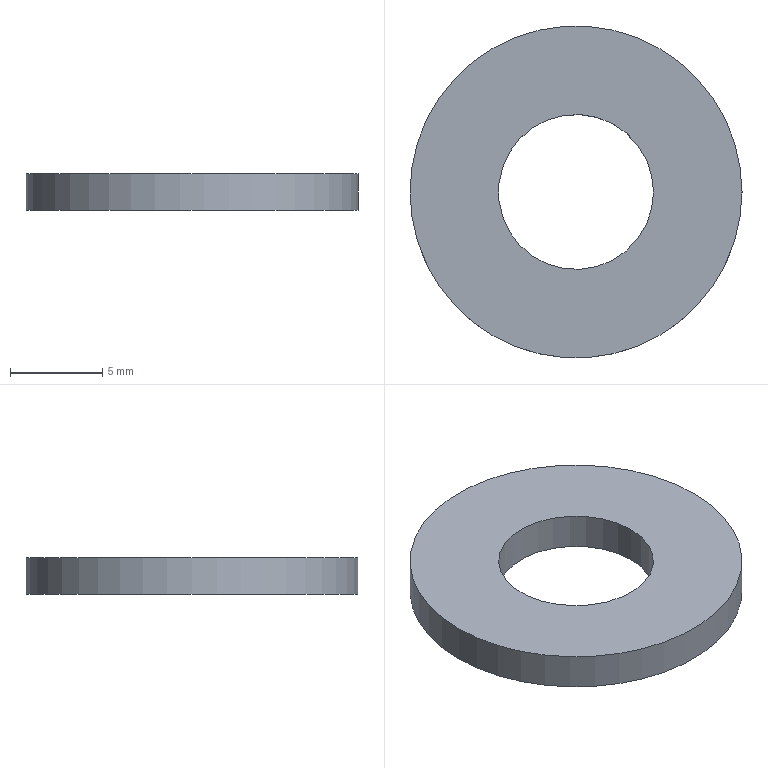Part | STEP file | 冲床-300配套压波_id94_x_t | 1 solid | 4 faces | box 18 x 18 x 2 mm | volume 398.103 mm3 | cylinder 2 | plane 2 | commonest cylinder face diameters 8.4 x1 18 x1
STEP:
#1=CARTESIAN_POINT('',(1174.,-205.,22.));
#2=VERTEX_POINT('',#1);
#3=CARTESIAN_POINT('',(1165.,-205.,22.));
#4=DIRECTION('',(0.,0.,1.));
#5=DIRECTION('',(1.,0.,0.));
#6=AXIS2_PLACEMENT_3D('',#3,#4,#5);
#7=CIRCLE('',#6,9.);
#8=EDGE_CURVE('',#2,#2,#7,.T.);
#9=ORIENTED_EDGE('',*,*,#8,.F.);
#10=EDGE_LOOP('',(#9));
#11=FACE_BOUND('',#10,.T.);
#12=CARTESIAN_POINT('',(1174.,-205.,20.));
#13=VERTEX_POINT('',#12);
#14=CARTESIAN_POINT('',(1165.,-205.,20.));
#15=DIRECTION('',(0.,0.,1.));
#16=DIRECTION('',(1.,0.,0.));
#17=AXIS2_PLACEMENT_3D('',#14,#15,#16);
#18=CIRCLE('',#17,9.);
#19=EDGE_CURVE('',#13,#13,#18,.T.);
#20=ORIENTED_EDGE('',*,*,#19,.T.);
#21=EDGE_LOOP('',(#20));
#22=FACE_BOUND('',#21,.T.);
#23=CARTESIAN_POINT('',(1165.,-205.,22.));
#24=DIRECTION('',(0.,0.,-1.));
#25=DIRECTION('',(-1.,0.,0.));
#26=AXIS2_PLACEMENT_3D('',#23,#24,#25);
#27=CYLINDRICAL_SURFACE('',#26,9.);
#28=ADVANCED_FACE('',(#11,#22),#27,.T.);
#29=CARTESIAN_POINT('',(1169.2,-205.,22.));
#30=VERTEX_POINT('',#29);
#31=CARTESIAN_POINT('',(1165.,-205.,22.));
#32=DIRECTION('',(0.,0.,1.));
#33=DIRECTION('',(1.,0.,0.));
#34=AXIS2_PLACEMENT_3D('',#31,#32,#33);
#35=CIRCLE('',#34,4.2);
#36=EDGE_CURVE('',#30,#30,#35,.T.);
#37=ORIENTED_EDGE('',*,*,#36,.T.);
#38=EDGE_LOOP('',(#37));
#39=FACE_BOUND('',#38,.T.);
#40=CARTESIAN_POINT('',(1169.2,-205.,20.));
#41=VERTEX_POINT('',#40);
#42=CARTESIAN_POINT('',(1165.,-205.,20.));
#43=DIRECTION('',(0.,0.,1.));
#44=DIRECTION('',(1.,0.,0.));
#45=AXIS2_PLACEMENT_3D('',#42,#43,#44);
#46=CIRCLE('',#45,4.2);
#47=EDGE_CURVE('',#41,#41,#46,.T.);
#48=ORIENTED_EDGE('',*,*,#47,.F.);
#49=EDGE_LOOP('',(#48));
#50=FACE_BOUND('',#49,.T.);
#51=CARTESIAN_POINT('',(1165.,-205.,22.));
#52=DIRECTION('',(0.,0.,-1.));
#53=DIRECTION('',(-1.,0.,0.));
#54=AXIS2_PLACEMENT_3D('',#51,#52,#53);
#55=CYLINDRICAL_SURFACE('',#54,4.2);
#56=ADVANCED_FACE('',(#39,#50),#55,.F.);
#57=ORIENTED_EDGE('',*,*,#8,.T.);
#58=EDGE_LOOP('',(#57));
#59=FACE_BOUND('',#58,.T.);
#60=ORIENTED_EDGE('',*,*,#36,.F.);
#61=EDGE_LOOP('',(#60));
#62=FACE_BOUND('',#61,.T.);
#63=CARTESIAN_POINT('',(1165.,-205.,22.));
#64=DIRECTION('',(0.,0.,1.));
#65=DIRECTION('',(1.,0.,0.));
#66=AXIS2_PLACEMENT_3D('',#63,#64,#65);
#67=PLANE('',#66);
#68=ADVANCED_FACE('',(#59,#62),#67,.T.);
#69=ORIENTED_EDGE('',*,*,#19,.F.);
#70=EDGE_LOOP('',(#69));
#71=FACE_BOUND('',#70,.T.);
#72=ORIENTED_EDGE('',*,*,#47,.T.);
#73=EDGE_LOOP('',(#72));
#74=FACE_BOUND('',#73,.T.);
#75=CARTESIAN_POINT('',(1165.,-205.,20.));
#76=DIRECTION('',(0.,0.,1.));
#77=DIRECTION('',(1.,0.,0.));
#78=AXIS2_PLACEMENT_3D('',#75,#76,#77);
#79=PLANE('',#78);
#80=ADVANCED_FACE('',(#71,#74),#79,.F.);
#81=CLOSED_SHELL('',(#28,#56,#68,#80));
#82=MANIFOLD_SOLID_BREP('',#81);
#83=(LENGTH_UNIT()NAMED_UNIT(*)SI_UNIT(.MILLI.,.METRE.));
#84=UNCERTAINTY_MEASURE_WITH_UNIT(LENGTH_MEASURE(0.00002),#83,'','');
#85=(NAMED_UNIT(*)PLANE_ANGLE_UNIT()SI_UNIT($,.RADIAN.));
#86=PLANE_ANGLE_MEASURE_WITH_UNIT(PLANE_ANGLE_MEASURE(0.01745),#85);
#87=DIMENSIONAL_EXPONENTS(0.,0.,0.,0.,0.,0.,0.);
#88=(CONVERSION_BASED_UNIT('DEGREE',#86)NAMED_UNIT(#87)PLANE_ANGLE_UNIT());
#89=(NAMED_UNIT(*)SI_UNIT($,.STERADIAN.)SOLID_ANGLE_UNIT());
#90=(GEOMETRIC_REPRESENTATION_CONTEXT(3)GLOBAL_UNCERTAINTY_ASSIGNED_CONTEXT((#84))GLOBAL_UNIT_ASSIGNED_CONTEXT((#83,#88,#89))REPRESENTATION_CONTEXT('',''));
#91=ADVANCED_BREP_SHAPE_REPRESENTATION('',(#82),#90);